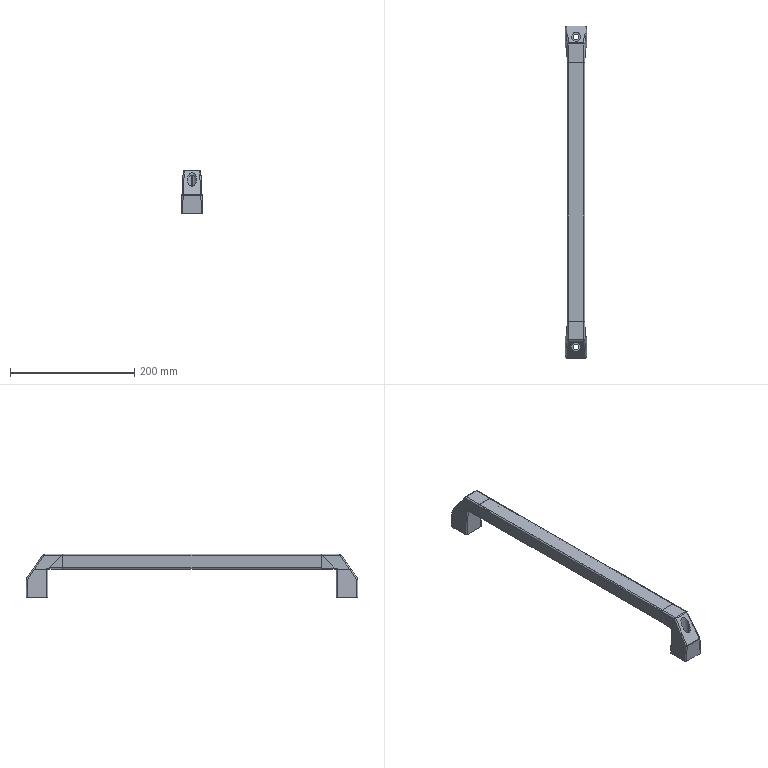Part | NX | features BREP 3 | 3 solids | 193 faces | box 35.311 x 535.2 x 70.2 mm | volume 135109 mm3 | plane 112 | cylinder 60 | sphere 19 | spline 2 | commonest cylinder face diameters 4 x42 18 x8 9 x4 15 x4 4.2 x2